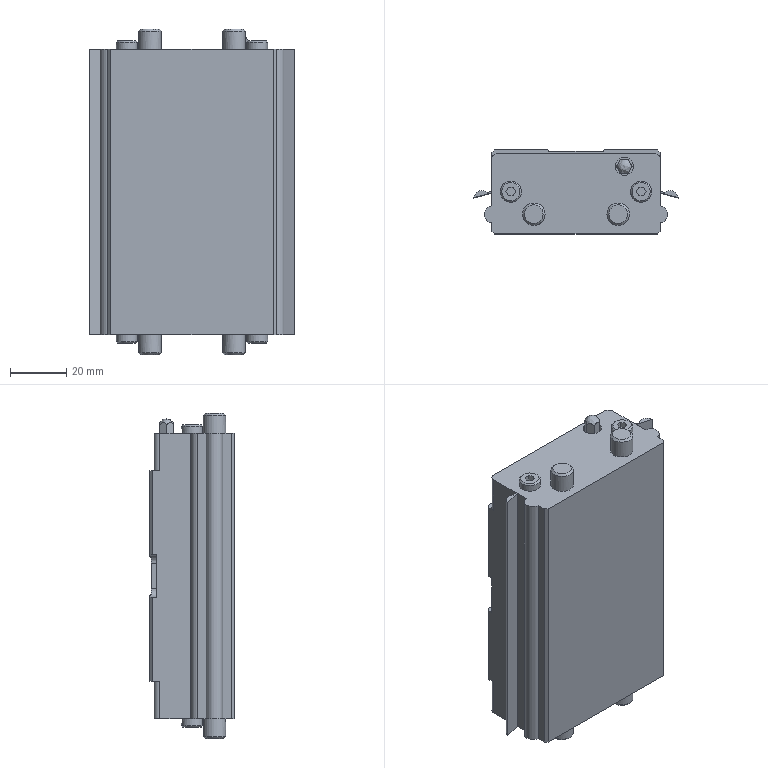Part | NX | 1 solid | 129 faces | box 72.933 x 30 x 116 mm | volume 182952 mm3 | plane 91 | cylinder 29 | cone 8 | spline 1 | commonest cylinder face diameters 6 x8 4 x4 5 x4 7.5 x4 8 x4 2.15 x2